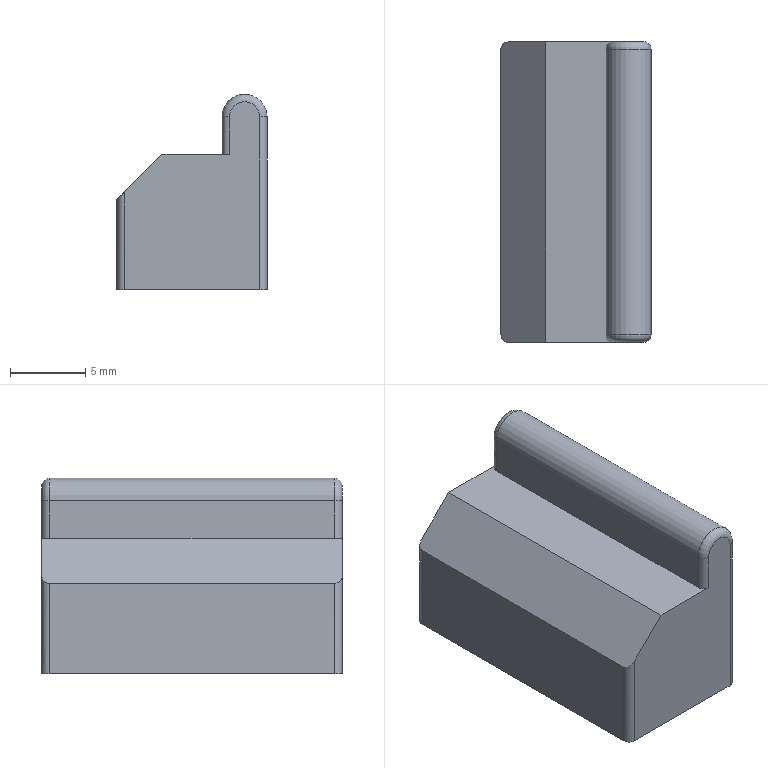CAM job | Mastercam | 3-axis milling, 5-axis milling, drilling | part box 10 x 20 x 13 mm | stock box 15 x 25 x 13 mm
Tools:
tool_number,name,type,diameter_mm,corner_radius_mm,flutes,flute_length_mm,overall_length_mm,shoulder_length_mm,holder_diameter_mm,length_offset,diameter_offset,default_rpm,default_feed_mm_min,default_plunge_mm_min,coolant
5,4 Chamfer Mill,chamfer mill,4,0,4,25,75,30,50,5,5,6250,750,600,COOL_OFF
9,10 Flat End Mill,end mill,10,0,4,25,75,25,50,9,9,1000,120,600,COOL_OFF
10,10 Flat End Mill,end mill,10,0,4,25,75,25,50,10,10,1000,120,600,COOL_OFF
14,4 Ball Mill / Bull Nose Mill,ball end mill,4,2,4,25,100,30,50,14,14,3000,360,600,COOL_OFF
18,8 Bull Nose Mill,bull end mill,8,1,4,25,100,25,50,18,18,1500,180,600,COOL_OFF
24,100 Flat End Mill,end mill,100,0,4,25,75,25,50,24,24,100,12,600,COOL_OFF
Operations:
seq,operation,operation_type,tool_number,tool_name,tool_diameter_mm,spindle_rpm,feed_mm_min,plunge_mm_min,retract_mm_min,cycle_time_s,wcs,posted,nc_file
1,Facing - [WCS: Plane] - [Tplane: Plane],Facing,24,100 Flat End Mill,100,4000,4000,600,1200,25.783,Plane,yes,.nc
2,Contour (Ramp) - [WCS: Plane] - [Tplane: Plane],Contour,9,10 Flat End Mill,10,8000,4000,600,1200,20.678,Plane,yes,.nc
3,Contour (2D) - [WCS: Plane] - [Tplane: Plane],Contour,10,10 Flat End Mill,10,6000,1000,600,1200,7.882,Plane,yes,.nc
4,Drill/Counterbore - [WCS: Plane] - [Tplane: Plane],Drill,5,4 Chamfer Mill,4,6000,200,600,1200,1.977,Plane,yes,.nc
5,Contour (2D chamfer) - [WCS: Plane] - [Tplane: Plane],Contour,5,4 Chamfer Mill,4,6000,1000,600,1200,4.649,Plane,yes,.nc
6,Facing - [WCS: Plane-1] - [Tplane: Plane-1],Facing,24,100 Flat End Mill,100,4000,4000,600,1200,25.783,Plane-1,yes,.nc
7,Contour (Ramp) - [WCS: Plane-1] - [Tplane: Plane-1],Contour,9,10 Flat End Mill,10,8000,3500,600,1200,5.482,Plane-1,yes,.nc
8,Contour (2D) - [WCS: Plane-1] - [Tplane: Plane-1],Contour,10,10 Flat End Mill,10,6000,1000,600,1200,3.6,Plane-1,yes,.nc
9,Surface Finish Flowline - [WCS: Plane-1] - [Tplane: Plane-1],MultiSurfaceFinishFlowline,18,8 Bull Nose Mill,8,8000,4000,600,1200,19.552,Plane-1,yes,.nc
10,Surface Finish Flowline - [WCS: Plane-1] - [Tplane: Plane-1],MultiSurfaceFinishFlowline,18,8 Bull Nose Mill,8,8000,4000,600,1200,25.342,Plane-1,yes,.nc
11,Unified Morph - [WCS: Plane-1] - [Tplane: Plane-1],461,14,4 Ball Mill / Bull Nose Mill,4,7000,3000,600,1200,3.729,Plane-1,yes,.nc
12,Unified Morph - [WCS: Plane-1] - [Tplane: Plane-1],461,14,4 Ball Mill / Bull Nose Mill,4,7000,3000,600,1200,3.729,Plane-1,yes,.nc
13,Deburr 5-axis - [WCS: Plane-1] - [Tplane: Plane-1],459,14,4 Ball Mill / Bull Nose Mill,4,7000,1000,600,1200,4.028,Plane-1,yes,.nc
14,Drill/Counterbore - [WCS: Plane-2] - [Tplane: Plane-2],Drill,5,4 Chamfer Mill,4,6000,200,600,1200,0.989,Plane-2,yes,.nc
15,Drill/Counterbore - [WCS: Plane-3] - [Tplane: Plane-3],Drill,5,4 Chamfer Mill,4,6000,200,600,1200,0.989,Plane-3,yes,.nc